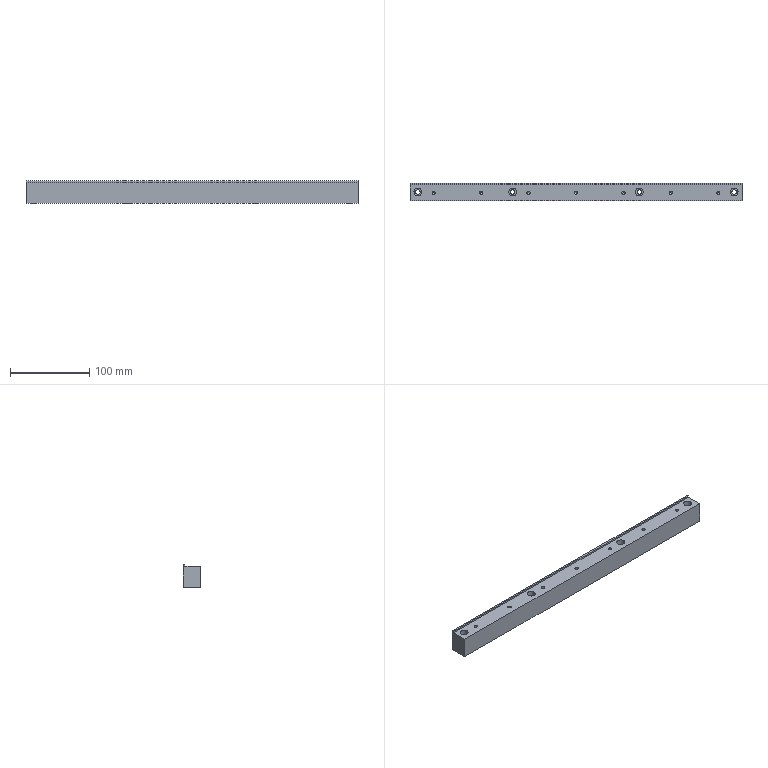Part | SolidWorks | features HoleWzd 2, Extrusion 1, ICE 1 | 1 solid | 56 faces | box 420 x 22 x 29 mm | volume 243626 mm3 | cylinder 30 | cone 14 | plane 12 | commonest cylinder face diameters 4.2 x14 5.5 x8 10 x8
STEP:
#1=CARTESIAN_POINT('',(195.,0.,10.));
#2=VERTEX_POINT('',#1);
#3=CARTESIAN_POINT('',(205.,0.,10.));
#4=VERTEX_POINT('',#3);
#5=CARTESIAN_POINT('',(200.,0.,10.));
#6=DIRECTION('',(0.,0.,1.));
#7=DIRECTION('',(1.,0.,0.));
#8=AXIS2_PLACEMENT_3D('',#5,#6,#7);
#9=CIRCLE('',#8,5.);
#10=EDGE_CURVE('',#2,#4,#9,.T.);
#11=ORIENTED_EDGE('',*,*,#10,.F.);
#12=CARTESIAN_POINT('',(195.,0.,27.));
#13=VERTEX_POINT('',#12);
#14=CARTESIAN_POINT('',(195.,0.,27.));
#15=DIRECTION('',(0.,0.,1.));
#16=VECTOR('',#15,1000.);
#17=LINE('',#14,#16);
#18=EDGE_CURVE('',#2,#13,#17,.T.);
#19=ORIENTED_EDGE('',*,*,#18,.T.);
#20=CARTESIAN_POINT('',(205.,0.,27.));
#21=VERTEX_POINT('',#20);
#22=CARTESIAN_POINT('',(200.,0.,27.));
#23=DIRECTION('',(0.,0.,1.));
#24=DIRECTION('',(1.,0.,0.));
#25=AXIS2_PLACEMENT_3D('',#22,#23,#24);
#26=CIRCLE('',#25,5.);
#27=EDGE_CURVE('',#13,#21,#26,.T.);
#28=ORIENTED_EDGE('',*,*,#27,.T.);
#29=CARTESIAN_POINT('',(205.,0.,27.));
#30=DIRECTION('',(0.,0.,1.));
#31=VECTOR('',#30,1000.);
#32=LINE('',#29,#31);
#33=EDGE_CURVE('',#4,#21,#32,.T.);
#34=ORIENTED_EDGE('',*,*,#33,.F.);
#35=EDGE_LOOP('',(#11,#19,#28,#34));
#36=FACE_OUTER_BOUND('',#35,.T.);
#37=CARTESIAN_POINT('',(200.,0.,27.));
#38=DIRECTION('',(0.,0.,1.));
#39=DIRECTION('',(1.,0.,0.));
#40=AXIS2_PLACEMENT_3D('',#37,#38,#39);
#41=CYLINDRICAL_SURFACE('',#40,5.);
#42=ADVANCED_FACE('',(#36),#41,.F.);
#43=CARTESIAN_POINT('',(197.25,0.,0.));
#44=VERTEX_POINT('',#43);
#45=CARTESIAN_POINT('',(202.75,0.,0.));
#46=VERTEX_POINT('',#45);
#47=CARTESIAN_POINT('',(200.,0.,0.));
#48=DIRECTION('',(0.,0.,1.));
#49=DIRECTION('',(1.,0.,0.));
#50=AXIS2_PLACEMENT_3D('',#47,#48,#49);
#51=CIRCLE('',#50,2.75);
#52=EDGE_CURVE('',#44,#46,#51,.T.);
#53=ORIENTED_EDGE('',*,*,#52,.F.);
#54=CARTESIAN_POINT('',(197.25,0.,10.));
#55=VERTEX_POINT('',#54);
#56=CARTESIAN_POINT('',(197.25,0.,27.));
#57=DIRECTION('',(0.,0.,1.));
#58=VECTOR('',#57,1000.);
#59=LINE('',#56,#58);
#60=EDGE_CURVE('',#44,#55,#59,.T.);
#61=ORIENTED_EDGE('',*,*,#60,.T.);
#62=CARTESIAN_POINT('',(202.75,0.,10.));
#63=VERTEX_POINT('',#62);
#64=CARTESIAN_POINT('',(200.,0.,10.));
#65=DIRECTION('',(0.,0.,1.));
#66=DIRECTION('',(1.,0.,0.));
#67=AXIS2_PLACEMENT_3D('',#64,#65,#66);
#68=CIRCLE('',#67,2.75);
#69=EDGE_CURVE('',#55,#63,#68,.T.);
#70=ORIENTED_EDGE('',*,*,#69,.T.);
#71=CARTESIAN_POINT('',(202.75,0.,27.));
#72=DIRECTION('',(0.,0.,1.));
#73=VECTOR('',#72,1000.);
#74=LINE('',#71,#73);
#75=EDGE_CURVE('',#46,#63,#74,.T.);
#76=ORIENTED_EDGE('',*,*,#75,.F.);
#77=EDGE_LOOP('',(#53,#61,#70,#76));
#78=FACE_OUTER_BOUND('',#77,.T.);
#79=CARTESIAN_POINT('',(200.,0.,27.));
#80=DIRECTION('',(0.,0.,1.));
#81=DIRECTION('',(1.,0.,0.));
#82=AXIS2_PLACEMENT_3D('',#79,#80,#81);
#83=CYLINDRICAL_SURFACE('',#82,2.75);
#84=ADVANCED_FACE('',(#78),#83,.F.);
#85=CARTESIAN_POINT('',(75.,0.,10.));
#86=VERTEX_POINT('',#85);
#87=CARTESIAN_POINT('',(85.,0.,10.));
#88=VERTEX_POINT('',#87);
#89=CARTESIAN_POINT('',(80.,0.,10.));
#90=DIRECTION('',(0.,0.,1.));
#91=DIRECTION('',(1.,0.,0.));
#92=AXIS2_PLACEMENT_3D('',#89,#90,#91);
#93=CIRCLE('',#92,5.);
#94=EDGE_CURVE('',#86,#88,#93,.T.);
#95=ORIENTED_EDGE('',*,*,#94,.F.);
#96=CARTESIAN_POINT('',(75.,0.,27.));
#97=VERTEX_POINT('',#96);
#98=CARTESIAN_POINT('',(75.,0.,27.));
#99=DIRECTION('',(0.,0.,1.));
#100=VECTOR('',#99,1000.);
#101=LINE('',#98,#100);
#102=EDGE_CURVE('',#86,#97,#101,.T.);
#103=ORIENTED_EDGE('',*,*,#102,.T.);
#104=CARTESIAN_POINT('',(85.,0.,27.));
#105=VERTEX_POINT('',#104);
#106=CARTESIAN_POINT('',(80.,0.,27.));
#107=DIRECTION('',(0.,0.,1.));
#108=DIRECTION('',(1.,0.,0.));
#109=AXIS2_PLACEMENT_3D('',#106,#107,#108);
#110=CIRCLE('',#109,5.);
#111=EDGE_CURVE('',#97,#105,#110,.T.);
#112=ORIENTED_EDGE('',*,*,#111,.T.);
#113=CARTESIAN_POINT('',(85.,0.,27.));
#114=DIRECTION('',(0.,0.,1.));
#115=VECTOR('',#114,1000.);
#116=LINE('',#113,#115);
#117=EDGE_CURVE('',#88,#105,#116,.T.);
#118=ORIENTED_EDGE('',*,*,#117,.F.);
#119=EDGE_LOOP('',(#95,#103,#112,#118));
#120=FACE_OUTER_BOUND('',#119,.T.);
#121=CARTESIAN_POINT('',(80.,0.,27.));
#122=DIRECTION('',(0.,0.,1.));
#123=DIRECTION('',(1.,0.,0.));
#124=AXIS2_PLACEMENT_3D('',#121,#122,#123);
#125=CYLINDRICAL_SURFACE('',#124,5.);
#126=ADVANCED_FACE('',(#120),#125,.F.);
#127=CARTESIAN_POINT('',(77.25,0.,0.));
#128=VERTEX_POINT('',#127);
#129=CARTESIAN_POINT('',(82.75,0.,0.));
#130=VERTEX_POINT('',#129);
#131=CARTESIAN_POINT('',(80.,0.,0.));
#132=DIRECTION('',(0.,0.,1.));
#133=DIRECTION('',(1.,0.,0.));
#134=AXIS2_PLACEMENT_3D('',#131,#132,#133);
#135=CIRCLE('',#134,2.75);
#136=EDGE_CURVE('',#128,#130,#135,.T.);
#137=ORIENTED_EDGE('',*,*,#136,.F.);
#138=CARTESIAN_POINT('',(77.25,0.,10.));
#139=VERTEX_POINT('',#138);
#140=CARTESIAN_POINT('',(77.25,0.,27.));
#141=DIRECTION('',(0.,0.,1.));
#142=VECTOR('',#141,1000.);
#143=LINE('',#140,#142);
#144=EDGE_CURVE('',#128,#139,#143,.T.);
#145=ORIENTED_EDGE('',*,*,#144,.T.);
#146=CARTESIAN_POINT('',(82.75,0.,10.));
#147=VERTEX_POINT('',#146);
#148=CARTESIAN_POINT('',(80.,0.,10.));
#149=DIRECTION('',(0.,0.,1.));
#150=DIRECTION('',(1.,0.,0.));
#151=AXIS2_PLACEMENT_3D('',#148,#149,#150);
#152=CIRCLE('',#151,2.75);
#153=EDGE_CURVE('',#139,#147,#152,.T.);
#154=ORIENTED_EDGE('',*,*,#153,.T.);
#155=CARTESIAN_POINT('',(82.75,0.,27.));
#156=DIRECTION('',(0.,0.,1.));
#157=VECTOR('',#156,1000.);
#158=LINE('',#155,#157);
#159=EDGE_CURVE('',#130,#147,#158,.T.);
#160=ORIENTED_EDGE('',*,*,#159,.F.);
#161=EDGE_LOOP('',(#137,#145,#154,#160));
#162=FACE_OUTER_BOUND('',#161,.T.);
#163=CARTESIAN_POINT('',(80.,0.,27.));
#164=DIRECTION('',(0.,0.,1.));
#165=DIRECTION('',(1.,0.,0.));
#166=AXIS2_PLACEMENT_3D('',#163,#164,#165);
#167=CYLINDRICAL_SURFACE('',#166,2.75);
#168=ADVANCED_FACE('',(#162),#167,.F.);
#169=CARTESIAN_POINT('',(-85.,0.,10.));
#170=VERTEX_POINT('',#169);
#171=CARTESIAN_POINT('',(-75.,0.,10.));
#172=VERTEX_POINT('',#171);
#173=CARTESIAN_POINT('',(-80.,0.,10.));
#174=DIRECTION('',(0.,0.,1.));
#175=DIRECTION('',(1.,0.,0.));
#176=AXIS2_PLACEMENT_3D('',#173,#174,#175);
#177=CIRCLE('',#176,5.);
#178=EDGE_CURVE('',#170,#172,#177,.T.);
#179=ORIENTED_EDGE('',*,*,#178,.F.);
#180=CARTESIAN_POINT('',(-85.,0.,27.));
#181=VERTEX_POINT('',#180);
#182=CARTESIAN_POINT('',(-85.,0.,27.));
#183=DIRECTION('',(0.,0.,1.));
#184=VECTOR('',#183,1000.);
#185=LINE('',#182,#184);
#186=EDGE_CURVE('',#170,#181,#185,.T.);
#187=ORIENTED_EDGE('',*,*,#186,.T.);
#188=CARTESIAN_POINT('',(-75.,0.,27.));
#189=VERTEX_POINT('',#188);
#190=CARTESIAN_POINT('',(-80.,0.,27.));
#191=DIRECTION('',(0.,0.,1.));
#192=DIRECTION('',(1.,0.,0.));
#193=AXIS2_PLACEMENT_3D('',#190,#191,#192);
#194=CIRCLE('',#193,5.);
#195=EDGE_CURVE('',#181,#189,#194,.T.);
#196=ORIENTED_EDGE('',*,*,#195,.T.);
#197=CARTESIAN_POINT('',(-75.,0.,27.));
#198=DIRECTION('',(0.,0.,1.));
#199=VECTOR('',#198,1000.);
#200=LINE('',#197,#199);
#201=EDGE_CURVE('',#172,#189,#200,.T.);
#202=ORIENTED_EDGE('',*,*,#201,.F.);
#203=EDGE_LOOP('',(#179,#187,#196,#202));
#204=FACE_OUTER_BOUND('',#203,.T.);
#205=CARTESIAN_POINT('',(-80.,0.,27.));
#206=DIRECTION('',(0.,0.,1.));
#207=DIRECTION('',(1.,0.,0.));
#208=AXIS2_PLACEMENT_3D('',#205,#206,#207);
#209=CYLINDRICAL_SURFACE('',#208,5.);
#210=ADVANCED_FACE('',(#204),#209,.F.);
#211=CARTESIAN_POINT('',(-82.75,0.,0.));
#212=VERTEX_POINT('',#211);
#213=CARTESIAN_POINT('',(-77.25,0.,0.));
#214=VERTEX_POINT('',#213);
#215=CARTESIAN_POINT('',(-80.,0.,0.));
#216=DIRECTION('',(0.,0.,1.));
#217=DIRECTION('',(1.,0.,0.));
#218=AXIS2_PLACEMENT_3D('',#215,#216,#217);
#219=CIRCLE('',#218,2.75);
#220=EDGE_CURVE('',#212,#214,#219,.T.);
#221=ORIENTED_EDGE('',*,*,#220,.F.);
#222=CARTESIAN_POINT('',(-82.75,0.,10.));
#223=VERTEX_POINT('',#222);
#224=CARTESIAN_POINT('',(-82.75,0.,27.));
#225=DIRECTION('',(0.,0.,1.));
#226=VECTOR('',#225,1000.);
#227=LINE('',#224,#226);
#228=EDGE_CURVE('',#212,#223,#227,.T.);
#229=ORIENTED_EDGE('',*,*,#228,.T.);
#230=CARTESIAN_POINT('',(-77.25,0.,10.));
#231=VERTEX_POINT('',#230);
#232=CARTESIAN_POINT('',(-80.,0.,10.));
#233=DIRECTION('',(0.,0.,1.));
#234=DIRECTION('',(1.,0.,0.));
#235=AXIS2_PLACEMENT_3D('',#232,#233,#234);
#236=CIRCLE('',#235,2.75);
#237=EDGE_CURVE('',#223,#231,#236,.T.);
#238=ORIENTED_EDGE('',*,*,#237,.T.);
#239=CARTESIAN_POINT('',(-77.25,0.,27.));
#240=DIRECTION('',(0.,0.,1.));
#241=VECTOR('',#240,1000.);
#242=LINE('',#239,#241);
#243=EDGE_CURVE('',#214,#231,#242,.T.);
#244=ORIENTED_EDGE('',*,*,#243,.F.);
#245=EDGE_LOOP('',(#221,#229,#238,#244));
#246=FACE_OUTER_BOUND('',#245,.T.);
#247=CARTESIAN_POINT('',(-80.,0.,27.));
#248=DIRECTION('',(0.,0.,1.));
#249=DIRECTION('',(1.,0.,0.));
#250=AXIS2_PLACEMENT_3D('',#247,#248,#249);
#251=CYLINDRICAL_SURFACE('',#250,2.75);
#252=ADVANCED_FACE('',(#246),#251,.F.);
#253=CARTESIAN_POINT('',(-205.,0.,10.));
#254=VERTEX_POINT('',#253);
#255=CARTESIAN_POINT('',(-195.,0.,10.));
#256=VERTEX_POINT('',#255);
#257=CARTESIAN_POINT('',(-200.,0.,10.));
#258=DIRECTION('',(0.,0.,1.));
#259=DIRECTION('',(1.,0.,0.));
#260=AXIS2_PLACEMENT_3D('',#257,#258,#259);
#261=CIRCLE('',#260,5.);
#262=EDGE_CURVE('',#254,#256,#261,.T.);
#263=ORIENTED_EDGE('',*,*,#262,.F.);
#264=CARTESIAN_POINT('',(-205.,0.,27.));
#265=VERTEX_POINT('',#264);
#266=CARTESIAN_POINT('',(-205.,0.,27.));
#267=DIRECTION('',(0.,0.,1.));
#268=VECTOR('',#267,1000.);
#269=LINE('',#266,#268);
#270=EDGE_CURVE('',#254,#265,#269,.T.);
#271=ORIENTED_EDGE('',*,*,#270,.T.);
#272=CARTESIAN_POINT('',(-195.,0.,27.));
#273=VERTEX_POINT('',#272);
#274=CARTESIAN_POINT('',(-200.,0.,27.));
#275=DIRECTION('',(0.,0.,1.));
#276=DIRECTION('',(1.,0.,0.));
#277=AXIS2_PLACEMENT_3D('',#274,#275,#276);
#278=CIRCLE('',#277,5.);
#279=EDGE_CURVE('',#265,#273,#278,.T.);
#280=ORIENTED_EDGE('',*,*,#279,.T.);
#281=CARTESIAN_POINT('',(-195.,0.,27.));
#282=DIRECTION('',(0.,0.,1.));
#283=VECTOR('',#282,1000.);
#284=LINE('',#281,#283);
#285=EDGE_CURVE('',#256,#273,#284,.T.);
#286=ORIENTED_EDGE('',*,*,#285,.F.);
#287=EDGE_LOOP('',(#263,#271,#280,#286));
#288=FACE_OUTER_BOUND('',#287,.T.);
#289=CARTESIAN_POINT('',(-200.,0.,27.));
#290=DIRECTION('',(0.,0.,1.));
#291=DIRECTION('',(1.,0.,0.));
#292=AXIS2_PLACEMENT_3D('',#289,#290,#291);
#293=CYLINDRICAL_SURFACE('',#292,5.);
#294=ADVANCED_FACE('',(#288),#293,.F.);
#295=CARTESIAN_POINT('',(-202.75,0.,0.));
#296=VERTEX_POINT('',#295);
#297=CARTESIAN_POINT('',(-197.25,0.,0.));
#298=VERTEX_POINT('',#297);
#299=CARTESIAN_POINT('',(-200.,0.,0.));
#300=DIRECTION('',(0.,0.,1.));
#301=DIRECTION('',(1.,0.,0.));
#302=AXIS2_PLACEMENT_3D('',#299,#300,#301);
#303=CIRCLE('',#302,2.75);
#304=EDGE_CURVE('',#296,#298,#303,.T.);
#305=ORIENTED_EDGE('',*,*,#304,.F.);
#306=CARTESIAN_POINT('',(-202.75,0.,10.));
#307=VERTEX_POINT('',#306);
#308=CARTESIAN_POINT('',(-202.75,0.,27.));
#309=DIRECTION('',(0.,0.,1.));
#310=VECTOR('',#309,1000.);
#311=LINE('',#308,#310);
#312=EDGE_CURVE('',#296,#307,#311,.T.);
#313=ORIENTED_EDGE('',*,*,#312,.T.);
#314=CARTESIAN_POINT('',(-197.25,0.,10.));
#315=VERTEX_POINT('',#314);
#316=CARTESIAN_POINT('',(-200.,0.,10.));
#317=DIRECTION('',(0.,0.,1.));
#318=DIRECTION('',(1.,0.,0.));
#319=AXIS2_PLACEMENT_3D('',#316,#317,#318);
#320=CIRCLE('',#319,2.75);
#321=EDGE_CURVE('',#307,#315,#320,.T.);
#322=ORIENTED_EDGE('',*,*,#321,.T.);
#323=CARTESIAN_POINT('',(-197.25,0.,27.));
#324=DIRECTION('',(0.,0.,1.));
#325=VECTOR('',#324,1000.);
#326=LINE('',#323,#325);
#327=EDGE_CURVE('',#298,#315,#326,.T.);
#328=ORIENTED_EDGE('',*,*,#327,.F.);
#329=EDGE_LOOP('',(#305,#313,#322,#328));
#330=FACE_OUTER_BOUND('',#329,.T.);
#331=CARTESIAN_POINT('',(-200.,0.,27.));
#332=DIRECTION('',(0.,0.,1.));
#333=DIRECTION('',(1.,0.,0.));
#334=AXIS2_PLACEMENT_3D('',#331,#332,#333);
#335=CYLINDRICAL_SURFACE('',#334,2.75);
#336=ADVANCED_FACE('',(#330),#335,.F.);
#337=CARTESIAN_POINT('',(177.9,-1.,14.6));
#338=VERTEX_POINT('',#337);
#339=CARTESIAN_POINT('',(182.1,-1.,14.6));
#340=VERTEX_POINT('',#339);
#341=CARTESIAN_POINT('',(180.,-1.,14.6));
#342=DIRECTION('',(0.,0.,1.));
#343=DIRECTION('',(1.,0.,0.));
#344=AXIS2_PLACEMENT_3D('',#341,#342,#343);
#345=CIRCLE('',#344,2.1);
#346=EDGE_CURVE('',#338,#340,#345,.T.);
#347=ORIENTED_EDGE('',*,*,#346,.F.);
#348=CARTESIAN_POINT('',(177.9,-1.,27.));
#349=VERTEX_POINT('',#348);
#350=CARTESIAN_POINT('',(177.9,-1.,27.));
#351=DIRECTION('',(0.,0.,1.));
#352=VECTOR('',#351,1000.);
#353=LINE('',#350,#352);
#354=EDGE_CURVE('',#338,#349,#353,.T.);
#355=ORIENTED_EDGE('',*,*,#354,.T.);
#356=CARTESIAN_POINT('',(182.1,-1.,27.));
#357=VERTEX_POINT('',#356);
#358=CARTESIAN_POINT('',(180.,-1.,27.));
#359=DIRECTION('',(0.,0.,1.));
#360=DIRECTION('',(1.,0.,0.));
#361=AXIS2_PLACEMENT_3D('',#358,#359,#360);
#362=CIRCLE('',#361,2.1);
#363=EDGE_CURVE('',#349,#357,#362,.T.);
#364=ORIENTED_EDGE('',*,*,#363,.T.);
#365=CARTESIAN_POINT('',(182.1,-1.,27.));
#366=DIRECTION('',(0.,0.,1.));
#367=VECTOR('',#366,1000.);
#368=LINE('',#365,#367);
#369=EDGE_CURVE('',#340,#357,#368,.T.);
#370=ORIENTED_EDGE('',*,*,#369,.F.);
#371=EDGE_LOOP('',(#347,#355,#364,#370));
#372=FACE_OUTER_BOUND('',#371,.T.);
#373=CARTESIAN_POINT('',(180.,-1.,27.));
#374=DIRECTION('',(0.,0.,1.));
#375=DIRECTION('',(1.,0.,0.));
#376=AXIS2_PLACEMENT_3D('',#373,#374,#375);
#377=CYLINDRICAL_SURFACE('',#376,2.1);
#378=ADVANCED_FACE('',(#372),#377,.F.);
#379=CARTESIAN_POINT('',(180.,-1.,13.338));
#380=VERTEX_POINT('',#379);
#381=CARTESIAN_POINT('',(182.1,-1.,14.6));
#382=DIRECTION('',(0.8572,0.,0.515));
#383=VECTOR('',#382,1000.);
#384=LINE('',#381,#383);
#385=EDGE_CURVE('',#380,#340,#384,.T.);
#386=ORIENTED_EDGE('',*,*,#385,.F.);
#387=CARTESIAN_POINT('',(177.9,-1.,14.6));
#388=DIRECTION('',(-0.8572,0.,0.515));
#389=VECTOR('',#388,1000.);
#390=LINE('',#387,#389);
#391=EDGE_CURVE('',#380,#338,#390,.T.);
#392=ORIENTED_EDGE('',*,*,#391,.T.);
#393=ORIENTED_EDGE('',*,*,#346,.T.);
#394=EDGE_LOOP('',(#386,#392,#393));
#395=FACE_OUTER_BOUND('',#394,.T.);
#396=CARTESIAN_POINT('',(180.,-1.,14.6));
#397=DIRECTION('',(0.,0.,1.));
#398=DIRECTION('',(1.,0.,0.));
#399=AXIS2_PLACEMENT_3D('',#396,#397,#398);
#400=CONICAL_SURFACE('',#399,2.1,1.03);
#401=ADVANCED_FACE('',(#395),#400,.F.);
#402=CARTESIAN_POINT('',(117.9,-1.,14.6));
#403=VERTEX_POINT('',#402);
#404=CARTESIAN_POINT('',(122.1,-1.,14.6));
#405=VERTEX_POINT('',#404);
#406=CARTESIAN_POINT('',(120.,-1.,14.6));
#407=DIRECTION('',(0.,0.,1.));
#408=DIRECTION('',(1.,0.,0.));
#409=AXIS2_PLACEMENT_3D('',#406,#407,#408);
#410=CIRCLE('',#409,2.1);
#411=EDGE_CURVE('',#403,#405,#410,.T.);
#412=ORIENTED_EDGE('',*,*,#411,.F.);
#413=CARTESIAN_POINT('',(117.9,-1.,27.));
#414=VERTEX_POINT('',#413);
#415=CARTESIAN_POINT('',(117.9,-1.,27.));
#416=DIRECTION('',(0.,0.,1.));
#417=VECTOR('',#416,1000.);
#418=LINE('',#415,#417);
#419=EDGE_CURVE('',#403,#414,#418,.T.);
#420=ORIENTED_EDGE('',*,*,#419,.T.);
#421=CARTESIAN_POINT('',(122.1,-1.,27.));
#422=VERTEX_POINT('',#421);
#423=CARTESIAN_POINT('',(120.,-1.,27.));
#424=DIRECTION('',(0.,0.,1.));
#425=DIRECTION('',(1.,0.,0.));
#426=AXIS2_PLACEMENT_3D('',#423,#424,#425);
#427=CIRCLE('',#426,2.1);
#428=EDGE_CURVE('',#414,#422,#427,.T.);
#429=ORIENTED_EDGE('',*,*,#428,.T.);
#430=CARTESIAN_POINT('',(122.1,-1.,27.));
#431=DIRECTION('',(0.,0.,1.));
#432=VECTOR('',#431,1000.);
#433=LINE('',#430,#432);
#434=EDGE_CURVE('',#405,#422,#433,.T.);
#435=ORIENTED_EDGE('',*,*,#434,.F.);
#436=EDGE_LOOP('',(#412,#420,#429,#435));
#437=FACE_OUTER_BOUND('',#436,.T.);
#438=CARTESIAN_POINT('',(120.,-1.,27.));
#439=DIRECTION('',(0.,0.,1.));
#440=DIRECTION('',(1.,0.,0.));
#441=AXIS2_PLACEMENT_3D('',#438,#439,#440);
#442=CYLINDRICAL_SURFACE('',#441,2.1);
#443=ADVANCED_FACE('',(#437),#442,.F.);
#444=CARTESIAN_POINT('',(120.,-1.,13.338));
#445=VERTEX_POINT('',#444);
#446=CARTESIAN_POINT('',(122.1,-1.,14.6));
#447=DIRECTION('',(0.8572,0.,0.515));
#448=VECTOR('',#447,1000.);
#449=LINE('',#446,#448);
#450=EDGE_CURVE('',#445,#405,#449,.T.);
#451=ORIENTED_EDGE('',*,*,#450,.F.);
#452=CARTESIAN_POINT('',(117.9,-1.,14.6));
#453=DIRECTION('',(-0.8572,0.,0.515));
#454=VECTOR('',#453,1000.);
#455=LINE('',#452,#454);
#456=EDGE_CURVE('',#445,#403,#455,.T.);
#457=ORIENTED_EDGE('',*,*,#456,.T.);
#458=ORIENTED_EDGE('',*,*,#411,.T.);
#459=EDGE_LOOP('',(#451,#457,#458));
#460=FACE_OUTER_BOUND('',#459,.T.);
#461=CARTESIAN_POINT('',(120.,-1.,14.6));
#462=DIRECTION('',(0.,0.,1.));
#463=DIRECTION('',(1.,0.,0.));
#464=AXIS2_PLACEMENT_3D('',#461,#462,#463);
#465=CONICAL_SURFACE('',#464,2.1,1.03);
#466=ADVANCED_FACE('',(#460),#465,.F.);
#467=CARTESIAN_POINT('',(57.9,-1.,14.6));
#468=VERTEX_POINT('',#467);
#469=CARTESIAN_POINT('',(62.1,-1.,14.6));
#470=VERTEX_POINT('',#469);
#471=CARTESIAN_POINT('',(60.,-1.,14.6));
#472=DIRECTION('',(0.,0.,1.));
#473=DIRECTION('',(1.,0.,0.));
#474=AXIS2_PLACEMENT_3D('',#471,#472,#473);
#475=CIRCLE('',#474,2.1);
#476=EDGE_CURVE('',#468,#470,#475,.T.);
#477=ORIENTED_EDGE('',*,*,#476,.F.);
#478=CARTESIAN_POINT('',(57.9,-1.,27.));
#479=VERTEX_POINT('',#478);
#480=CARTESIAN_POINT('',(57.9,-1.,27.));
#481=DIRECTION('',(0.,0.,1.));
#482=VECTOR('',#481,1000.);
#483=LINE('',#480,#482);
#484=EDGE_CURVE('',#468,#479,#483,.T.);
#485=ORIENTED_EDGE('',*,*,#484,.T.);
#486=CARTESIAN_POINT('',(62.1,-1.,27.));
#487=VERTEX_POINT('',#486);
#488=CARTESIAN_POINT('',(60.,-1.,27.));
#489=DIRECTION('',(0.,0.,1.));
#490=DIRECTION('',(1.,0.,0.));
#491=AXIS2_PLACEMENT_3D('',#488,#489,#490);
#492=CIRCLE('',#491,2.1);
#493=EDGE_CURVE('',#479,#487,#492,.T.);
#494=ORIENTED_EDGE('',*,*,#493,.T.);
#495=CARTESIAN_POINT('',(62.1,-1.,27.));
#496=DIRECTION('',(0.,0.,1.));
#497=VECTOR('',#496,1000.);
#498=LINE('',#495,#497);
#499=EDGE_CURVE('',#470,#487,#498,.T.);
#500=ORIENTED_EDGE('',*,*,#499,.F.);
#501=EDGE_LOOP('',(#477,#485,#494,#500));
#502=FACE_OUTER_BOUND('',#501,.T.);
#503=CARTESIAN_POINT('',(60.,-1.,27.));
#504=DIRECTION('',(0.,0.,1.));
#505=DIRECTION('',(1.,0.,0.));
#506=AXIS2_PLACEMENT_3D('',#503,#504,#505);
#507=CYLINDRICAL_SURFACE('',#506,2.1);
#508=ADVANCED_FACE('',(#502),#507,.F.);
#509=CARTESIAN_POINT('',(60.,-1.,13.338));
#510=VERTEX_POINT('',#509);
#511=CARTESIAN_POINT('',(62.1,-1.,14.6));
#512=DIRECTION('',(0.8572,0.,0.515));
#513=VECTOR('',#512,1000.);
#514=LINE('',#511,#513);
#515=EDGE_CURVE('',#510,#470,#514,.T.);
#516=ORIENTED_EDGE('',*,*,#515,.F.);
#517=CARTESIAN_POINT('',(57.9,-1.,14.6));
#518=DIRECTION('',(-0.8572,0.,0.515));
#519=VECTOR('',#518,1000.);
#520=LINE('',#517,#519);
#521=EDGE_CURVE('',#510,#468,#520,.T.);
#522=ORIENTED_EDGE('',*,*,#521,.T.);
#523=ORIENTED_EDGE('',*,*,#476,.T.);
#524=EDGE_LOOP('',(#516,#522,#523));
#525=FACE_OUTER_BOUND('',#524,.T.);
#526=CARTESIAN_POINT('',(60.,-1.,14.6));
#527=DIRECTION('',(0.,0.,1.));
#528=DIRECTION('',(1.,0.,0.));
#529=AXIS2_PLACEMENT_3D('',#526,#527,#528);
#530=CONICAL_SURFACE('',#529,2.1,1.03);
#531=ADVANCED_FACE('',(#525),#530,.F.);
#532=CARTESIAN_POINT('',(-2.1,-1.,14.6));
#533=VERTEX_POINT('',#532);
#534=CARTESIAN_POINT('',(2.1,-1.,14.6));
#535=VERTEX_POINT('',#534);
#536=CARTESIAN_POINT('',(0.,-1.,14.6));
#537=DIRECTION('',(0.,0.,1.));
#538=DIRECTION('',(1.,0.,0.));
#539=AXIS2_PLACEMENT_3D('',#536,#537,#538);
#540=CIRCLE('',#539,2.1);
#541=EDGE_CURVE('',#533,#535,#540,.T.);
#542=ORIENTED_EDGE('',*,*,#541,.F.);
#543=CARTESIAN_POINT('',(-2.1,-1.,27.));
#544=VERTEX_POINT('',#543);
#545=CARTESIAN_POINT('',(-2.1,-1.,27.));
#546=DIRECTION('',(0.,0.,1.));
#547=VECTOR('',#546,1000.);
#548=LINE('',#545,#547);
#549=EDGE_CURVE('',#533,#544,#548,.T.);
#550=ORIENTED_EDGE('',*,*,#549,.T.);
#551=CARTESIAN_POINT('',(2.1,-1.,27.));
#552=VERTEX_POINT('',#551);
#553=CARTESIAN_POINT('',(0.,-1.,27.));
#554=DIRECTION('',(0.,0.,1.));
#555=DIRECTION('',(1.,0.,0.));
#556=AXIS2_PLACEMENT_3D('',#553,#554,#555);
#557=CIRCLE('',#556,2.1);
#558=EDGE_CURVE('',#544,#552,#557,.T.);
#559=ORIENTED_EDGE('',*,*,#558,.T.);
#560=CARTESIAN_POINT('',(2.1,-1.,27.));
#561=DIRECTION('',(0.,0.,1.));
#562=VECTOR('',#561,1000.);
#563=LINE('',#560,#562);
#564=EDGE_CURVE('',#535,#552,#563,.T.);
#565=ORIENTED_EDGE('',*,*,#564,.F.);
#566=EDGE_LOOP('',(#542,#550,#559,#565));
#567=FACE_OUTER_BOUND('',#566,.T.);
#568=CARTESIAN_POINT('',(0.,-1.,27.));
#569=DIRECTION('',(0.,0.,1.));
#570=DIRECTION('',(1.,0.,0.));
#571=AXIS2_PLACEMENT_3D('',#568,#569,#570);
#572=CYLINDRICAL_SURFACE('',#571,2.1);
#573=ADVANCED_FACE('',(#567),#572,.F.);
#574=CARTESIAN_POINT('',(0.,-1.,13.338));
#575=VERTEX_POINT('',#574);
#576=CARTESIAN_POINT('',(2.1,-1.,14.6));
#577=DIRECTION('',(0.8572,0.,0.515));
#578=VECTOR('',#577,1000.);
#579=LINE('',#576,#578);
#580=EDGE_CURVE('',#575,#535,#579,.T.);
#581=ORIENTED_EDGE('',*,*,#580,.F.);
#582=CARTESIAN_POINT('',(-2.1,-1.,14.6));
#583=DIRECTION('',(-0.8572,0.,0.515));
#584=VECTOR('',#583,1000.);
#585=LINE('',#582,#584);
#586=EDGE_CURVE('',#575,#533,#585,.T.);
#587=ORIENTED_EDGE('',*,*,#586,.T.);
#588=ORIENTED_EDGE('',*,*,#541,.T.);
#589=EDGE_LOOP('',(#581,#587,#588));
#590=FACE_OUTER_BOUND('',#589,.T.);
#591=CARTESIAN_POINT('',(0.,-1.,14.6));
#592=DIRECTION('',(0.,0.,1.));
#593=DIRECTION('',(1.,0.,0.));
#594=AXIS2_PLACEMENT_3D('',#591,#592,#593);
#595=CONICAL_SURFACE('',#594,2.1,1.03);
#596=ADVANCED_FACE('',(#590),#595,.F.);
#597=CARTESIAN_POINT('',(-182.1,-1.,14.6));
#598=VERTEX_POINT('',#597);
#599=CARTESIAN_POINT('',(-177.9,-1.,14.6));
#600=VERTEX_POINT('',#599);
#601=CARTESIAN_POINT('',(-180.,-1.,14.6));
#602=DIRECTION('',(0.,0.,1.));
#603=DIRECTION('',(1.,0.,0.));
#604=AXIS2_PLACEMENT_3D('',#601,#602,#603);
#605=CIRCLE('',#604,2.1);
#606=EDGE_CURVE('',#598,#600,#605,.T.);
#607=ORIENTED_EDGE('',*,*,#606,.F.);
#608=CARTESIAN_POINT('',(-182.1,-1.,27.));
#609=VERTEX_POINT('',#608);
#610=CARTESIAN_POINT('',(-182.1,-1.,27.));
#611=DIRECTION('',(0.,0.,1.));
#612=VECTOR('',#611,1000.);
#613=LINE('',#610,#612);
#614=EDGE_CURVE('',#598,#609,#613,.T.);
#615=ORIENTED_EDGE('',*,*,#614,.T.);
#616=CARTESIAN_POINT('',(-177.9,-1.,27.));
#617=VERTEX_POINT('',#616);
#618=CARTESIAN_POINT('',(-180.,-1.,27.));
#619=DIRECTION('',(0.,0.,1.));
#620=DIRECTION('',(1.,0.,0.));
#621=AXIS2_PLACEMENT_3D('',#618,#619,#620);
#622=CIRCLE('',#621,2.1);
#623=EDGE_CURVE('',#609,#617,#622,.T.);
#624=ORIENTED_EDGE('',*,*,#623,.T.);
#625=CARTESIAN_POINT('',(-177.9,-1.,27.));
#626=DIRECTION('',(0.,0.,1.));
#627=VECTOR('',#626,1000.);
#628=LINE('',#625,#627);
#629=EDGE_CURVE('',#600,#617,#628,.T.);
#630=ORIENTED_EDGE('',*,*,#629,.F.);
#631=EDGE_LOOP('',(#607,#615,#624,#630));
#632=FACE_OUTER_BOUND('',#631,.T.);
#633=CARTESIAN_POINT('',(-180.,-1.,27.));
#634=DIRECTION('',(0.,0.,1.));
#635=DIRECTION('',(1.,0.,0.));
#636=AXIS2_PLACEMENT_3D('',#633,#634,#635);
#637=CYLINDRICAL_SURFACE('',#636,2.1);
#638=ADVANCED_FACE('',(#632),#637,.F.);
#639=CARTESIAN_POINT('',(-180.,-1.,13.338));
#640=VERTEX_POINT('',#639);
#641=CARTESIAN_POINT('',(-177.9,-1.,14.6));
#642=DIRECTION('',(0.8572,0.,0.515));
#643=VECTOR('',#642,1000.);
#644=LINE('',#641,#643);
#645=EDGE_CURVE('',#640,#600,#644,.T.);
#646=ORIENTED_EDGE('',*,*,#645,.F.);
#647=CARTESIAN_POINT('',(-182.1,-1.,14.6));
#648=DIRECTION('',(-0.8572,0.,0.515));
#649=VECTOR('',#648,1000.);
#650=LINE('',#647,#649);
#651=EDGE_CURVE('',#640,#598,#650,.T.);
#652=ORIENTED_EDGE('',*,*,#651,.T.);
#653=ORIENTED_EDGE('',*,*,#606,.T.);
#654=EDGE_LOOP('',(#646,#652,#653));
#655=FACE_OUTER_BOUND('',#654,.T.);
#656=CARTESIAN_POINT('',(-180.,-1.,14.6));
#657=DIRECTION('',(0.,0.,1.));
#658=DIRECTION('',(1.,0.,0.));
#659=AXIS2_PLACEMENT_3D('',#656,#657,#658);
#660=CONICAL_SURFACE('',#659,2.1,1.03);
#661=ADVANCED_FACE('',(#655),#660,.F.);
#662=CARTESIAN_POINT('',(-122.1,-1.,14.6));
#663=VERTEX_POINT('',#662);
#664=CARTESIAN_POINT('',(-117.9,-1.,14.6));
#665=VERTEX_POINT('',#664);
#666=CARTESIAN_POINT('',(-120.,-1.,14.6));
#667=DIRECTION('',(0.,0.,1.));
#668=DIRECTION('',(1.,0.,0.));
#669=AXIS2_PLACEMENT_3D('',#666,#667,#668);
#670=CIRCLE('',#669,2.1);
#671=EDGE_CURVE('',#663,#665,#670,.T.);
#672=ORIENTED_EDGE('',*,*,#671,.F.);
#673=CARTESIAN_POINT('',(-122.1,-1.,27.));
#674=VERTEX_POINT('',#673);
#675=CARTESIAN_POINT('',(-122.1,-1.,27.));
#676=DIRECTION('',(0.,0.,1.));
#677=VECTOR('',#676,1000.);
#678=LINE('',#675,#677);
#679=EDGE_CURVE('',#663,#674,#678,.T.);
#680=ORIENTED_EDGE('',*,*,#679,.T.);
#681=CARTESIAN_POINT('',(-117.9,-1.,27.));
#682=VERTEX_POINT('',#681);
#683=CARTESIAN_POINT('',(-120.,-1.,27.));
#684=DIRECTION('',(0.,0.,1.));
#685=DIRECTION('',(1.,0.,0.));
#686=AXIS2_PLACEMENT_3D('',#683,#684,#685);
#687=CIRCLE('',#686,2.1);
#688=EDGE_CURVE('',#674,#682,#687,.T.);
#689=ORIENTED_EDGE('',*,*,#688,.T.);
#690=CARTESIAN_POINT('',(-117.9,-1.,27.));
#691=DIRECTION('',(0.,0.,1.));
#692=VECTOR('',#691,1000.);
#693=LINE('',#690,#692);
#694=EDGE_CURVE('',#665,#682,#693,.T.);
#695=ORIENTED_EDGE('',*,*,#694,.F.);
#696=EDGE_LOOP('',(#672,#680,#689,#695));
#697=FACE_OUTER_BOUND('',#696,.T.);
#698=CARTESIAN_POINT('',(-120.,-1.,27.));
#699=DIRECTION('',(0.,0.,1.));
#700=DIRECTION('',(1.,0.,0.));
#701=AXIS2_PLACEMENT_3D('',#698,#699,#700);
#702=CYLINDRICAL_SURFACE('',#701,2.1);
#703=ADVANCED_FACE('',(#697),#702,.F.);
#704=CARTESIAN_POINT('',(-120.,-1.,13.338));
#705=VERTEX_POINT('',#704);
#706=CARTESIAN_POINT('',(-117.9,-1.,14.6));
#707=DIRECTION('',(0.8572,0.,0.515));
#708=VECTOR('',#707,1000.);
#709=LINE('',#706,#708);
#710=EDGE_CURVE('',#705,#665,#709,.T.);
#711=ORIENTED_EDGE('',*,*,#710,.F.);
#712=CARTESIAN_POINT('',(-122.1,-1.,14.6));
#713=DIRECTION('',(-0.8572,0.,0.515));
#714=VECTOR('',#713,1000.);
#715=LINE('',#712,#714);
#716=EDGE_CURVE('',#705,#663,#715,.T.);
#717=ORIENTED_EDGE('',*,*,#716,.T.);
#718=ORIENTED_EDGE('',*,*,#671,.T.);
#719=EDGE_LOOP('',(#711,#717,#718));
#720=FACE_OUTER_BOUND('',#719,.T.);
#721=CARTESIAN_POINT('',(-120.,-1.,14.6));
#722=DIRECTION('',(0.,0.,1.));
#723=DIRECTION('',(1.,0.,0.));
#724=AXIS2_PLACEMENT_3D('',#721,#722,#723);
#725=CONICAL_SURFACE('',#724,2.1,1.03);
#726=ADVANCED_FACE('',(#720),#725,.F.);
#727=CARTESIAN_POINT('',(-62.1,-1.,14.6));
#728=VERTEX_POINT('',#727);
#729=CARTESIAN_POINT('',(-57.9,-1.,14.6));
#730=VERTEX_POINT('',#729);
#731=CARTESIAN_POINT('',(-60.,-1.,14.6));
#732=DIRECTION('',(0.,0.,1.));
#733=DIRECTION('',(1.,0.,0.));
#734=AXIS2_PLACEMENT_3D('',#731,#732,#733);
#735=CIRCLE('',#734,2.1);
#736=EDGE_CURVE('',#728,#730,#735,.T.);
#737=ORIENTED_EDGE('',*,*,#736,.F.);
#738=CARTESIAN_POINT('',(-62.1,-1.,27.));
#739=VERTEX_POINT('',#738);
#740=CARTESIAN_POINT('',(-62.1,-1.,27.));
#741=DIRECTION('',(0.,0.,1.));
#742=VECTOR('',#741,1000.);
#743=LINE('',#740,#742);
#744=EDGE_CURVE('',#728,#739,#743,.T.);
#745=ORIENTED_EDGE('',*,*,#744,.T.);
#746=CARTESIAN_POINT('',(-57.9,-1.,27.));
#747=VERTEX_POINT('',#746);
#748=CARTESIAN_POINT('',(-60.,-1.,27.));
#749=DIRECTION('',(0.,0.,1.));
#750=DIRECTION('',(1.,0.,0.));
#751=AXIS2_PLACEMENT_3D('',#748,#749,#750);
#752=CIRCLE('',#751,2.1);
#753=EDGE_CURVE('',#739,#747,#752,.T.);
#754=ORIENTED_EDGE('',*,*,#753,.T.);
#755=CARTESIAN_POINT('',(-57.9,-1.,27.));
#756=DIRECTION('',(0.,0.,1.));
#757=VECTOR('',#756,1000.);
#758=LINE('',#755,#757);
#759=EDGE_CURVE('',#730,#747,#758,.T.);
#760=ORIENTED_EDGE('',*,*,#759,.F.);
#761=EDGE_LOOP('',(#737,#745,#754,#760));
#762=FACE_OUTER_BOUND('',#761,.T.);
#763=CARTESIAN_POINT('',(-60.,-1.,27.));
#764=DIRECTION('',(0.,0.,1.));
#765=DIRECTION('',(1.,0.,0.));
#766=AXIS2_PLACEMENT_3D('',#763,#764,#765);
#767=CYLINDRICAL_SURFACE('',#766,2.1);
#768=ADVANCED_FACE('',(#762),#767,.F.);
#769=CARTESIAN_POINT('',(-60.,-1.,13.338));
#770=VERTEX_POINT('',#769);
#771=CARTESIAN_POINT('',(-57.9,-1.,14.6));
#772=DIRECTION('',(0.8572,0.,0.515));
#773=VECTOR('',#772,1000.);
#774=LINE('',#771,#773);
#775=EDGE_CURVE('',#770,#730,#774,.T.);
#776=ORIENTED_EDGE('',*,*,#775,.F.);
#777=CARTESIAN_POINT('',(-62.1,-1.,14.6));
#778=DIRECTION('',(-0.8572,0.,0.515));
#779=VECTOR('',#778,1000.);
#780=LINE('',#777,#779);
#781=EDGE_CURVE('',#770,#728,#780,.T.);
#782=ORIENTED_EDGE('',*,*,#781,.T.);
#783=ORIENTED_EDGE('',*,*,#736,.T.);
#784=EDGE_LOOP('',(#776,#782,#783));
#785=FACE_OUTER_BOUND('',#784,.T.);
#786=CARTESIAN_POINT('',(-60.,-1.,14.6));
#787=DIRECTION('',(0.,0.,1.));
#788=DIRECTION('',(1.,0.,0.));
#789=AXIS2_PLACEMENT_3D('',#786,#787,#788);
#790=CONICAL_SURFACE('',#789,2.1,1.03);
#791=ADVANCED_FACE('',(#785),#790,.F.);
#792=CARTESIAN_POINT('',(200.,0.,27.));
#793=DIRECTION('',(0.,0.,1.));
#794=DIRECTION('',(1.,0.,0.));
#795=AXIS2_PLACEMENT_3D('',#792,#793,#794);
#796=CIRCLE('',#795,5.);
#797=EDGE_CURVE('',#21,#13,#796,.T.);
#798=ORIENTED_EDGE('',*,*,#797,.F.);
#799=ORIENTED_EDGE('',*,*,#27,.F.);
#800=EDGE_LOOP('',(#798,#799));
#801=FACE_BOUND('',#800,.T.);
#802=CARTESIAN_POINT('',(80.,0.,27.));
#803=DIRECTION('',(0.,0.,1.));
#804=DIRECTION('',(1.,0.,0.));
#805=AXIS2_PLACEMENT_3D('',#802,#803,#804);
#806=CIRCLE('',#805,5.);
#807=EDGE_CURVE('',#105,#97,#806,.T.);
#808=ORIENTED_EDGE('',*,*,#807,.F.);
#809=ORIENTED_EDGE('',*,*,#111,.F.);
#810=EDGE_LOOP('',(#808,#809));
#811=FACE_BOUND('',#810,.T.);
#812=CARTESIAN_POINT('',(-80.,0.,27.));
#813=DIRECTION('',(0.,0.,1.));
#814=DIRECTION('',(1.,0.,0.));
#815=AXIS2_PLACEMENT_3D('',#812,#813,#814);
#816=CIRCLE('',#815,5.);
#817=EDGE_CURVE('',#189,#181,#816,.T.);
#818=ORIENTED_EDGE('',*,*,#817,.F.);
#819=ORIENTED_EDGE('',*,*,#195,.F.);
#820=EDGE_LOOP('',(#818,#819));
#821=FACE_BOUND('',#820,.T.);
#822=CARTESIAN_POINT('',(-200.,0.,27.));
#823=DIRECTION('',(0.,0.,1.));
#824=DIRECTION('',(1.,0.,0.));
#825=AXIS2_PLACEMENT_3D('',#822,#823,#824);
#826=CIRCLE('',#825,5.);
#827=EDGE_CURVE('',#273,#265,#826,.T.);
#828=ORIENTED_EDGE('',*,*,#827,.F.);
#829=ORIENTED_EDGE('',*,*,#279,.F.);
#830=EDGE_LOOP('',(#828,#829));
#831=FACE_BOUND('',#830,.T.);
#832=CARTESIAN_POINT('',(180.,-1.,27.));
#833=DIRECTION('',(0.,0.,1.));
#834=DIRECTION('',(1.,0.,0.));
#835=AXIS2_PLACEMENT_3D('',#832,#833,#834);
#836=CIRCLE('',#835,2.1);
#837=EDGE_CURVE('',#357,#349,#836,.T.);
#838=ORIENTED_EDGE('',*,*,#837,.F.);
#839=ORIENTED_EDGE('',*,*,#363,.F.);
#840=EDGE_LOOP('',(#838,#839));
#841=FACE_BOUND('',#840,.T.);
#842=CARTESIAN_POINT('',(120.,-1.,27.));
#843=DIRECTION('',(0.,0.,1.));
#844=DIRECTION('',(1.,0.,0.));
#845=AXIS2_PLACEMENT_3D('',#842,#843,#844);
#846=CIRCLE('',#845,2.1);
#847=EDGE_CURVE('',#422,#414,#846,.T.);
#848=ORIENTED_EDGE('',*,*,#847,.F.);
#849=ORIENTED_EDGE('',*,*,#428,.F.);
#850=EDGE_LOOP('',(#848,#849));
#851=FACE_BOUND('',#850,.T.);
#852=CARTESIAN_POINT('',(60.,-1.,27.));
#853=DIRECTION('',(0.,0.,1.));
#854=DIRECTION('',(1.,0.,0.));
#855=AXIS2_PLACEMENT_3D('',#852,#853,#854);
#856=CIRCLE('',#855,2.1);
#857=EDGE_CURVE('',#487,#479,#856,.T.);
#858=ORIENTED_EDGE('',*,*,#857,.F.);
#859=ORIENTED_EDGE('',*,*,#493,.F.);
#860=EDGE_LOOP('',(#858,#859));
#861=FACE_BOUND('',#860,.T.);
#862=CARTESIAN_POINT('',(0.,-1.,27.));
#863=DIRECTION('',(0.,0.,1.));
#864=DIRECTION('',(1.,0.,0.));
#865=AXIS2_PLACEMENT_3D('',#862,#863,#864);
#866=CIRCLE('',#865,2.1);
#867=EDGE_CURVE('',#552,#544,#866,.T.);
#868=ORIENTED_EDGE('',*,*,#867,.F.);
#869=ORIENTED_EDGE('',*,*,#558,.F.);
#870=EDGE_LOOP('',(#868,#869));
#871=FACE_BOUND('',#870,.T.);
#872=CARTESIAN_POINT('',(-180.,-1.,27.));
#873=DIRECTION('',(0.,0.,1.));
#874=DIRECTION('',(1.,0.,0.));
#875=AXIS2_PLACEMENT_3D('',#872,#873,#874);
#876=CIRCLE('',#875,2.1);
#877=EDGE_CURVE('',#617,#609,#876,.T.);
#878=ORIENTED_EDGE('',*,*,#877,.F.);
#879=ORIENTED_EDGE('',*,*,#623,.F.);
#880=EDGE_LOOP('',(#878,#879));
#881=FACE_BOUND('',#880,.T.);
#882=CARTESIAN_POINT('',(-120.,-1.,27.));
#883=DIRECTION('',(0.,0.,1.));
#884=DIRECTION('',(1.,0.,0.));
#885=AXIS2_PLACEMENT_3D('',#882,#883,#884);
#886=CIRCLE('',#885,2.1);
#887=EDGE_CURVE('',#682,#674,#886,.T.);
#888=ORIENTED_EDGE('',*,*,#887,.F.);
#889=ORIENTED_EDGE('',*,*,#688,.F.);
#890=EDGE_LOOP('',(#888,#889));
#891=FACE_BOUND('',#890,.T.);
#892=CARTESIAN_POINT('',(-60.,-1.,27.));
#893=DIRECTION('',(0.,0.,1.));
#894=DIRECTION('',(1.,0.,0.));
#895=AXIS2_PLACEMENT_3D('',#892,#893,#894);
#896=CIRCLE('',#895,2.1);
#897=EDGE_CURVE('',#747,#739,#896,.T.);
#898=ORIENTED_EDGE('',*,*,#897,.F.);
#899=ORIENTED_EDGE('',*,*,#753,.F.);
#900=EDGE_LOOP('',(#898,#899));
#901=FACE_BOUND('',#900,.T.);
#902=CARTESIAN_POINT('',(-210.,9.,27.));
#903=VERTEX_POINT('',#902);
#904=CARTESIAN_POINT('',(210.,9.,27.));
#905=VERTEX_POINT('',#904);
#906=CARTESIAN_POINT('',(-210.,9.,27.));
#907=DIRECTION('',(1.,0.,0.));
#908=VECTOR('',#907,1000.);
#909=LINE('',#906,#908);
#910=EDGE_CURVE('',#903,#905,#909,.T.);
#911=ORIENTED_EDGE('',*,*,#910,.F.);
#912=CARTESIAN_POINT('',(-210.,-11.,27.));
#913=VERTEX_POINT('',#912);
#914=CARTESIAN_POINT('',(-210.,-11.,27.));
#915=DIRECTION('',(0.,-1.,0.));
#916=VECTOR('',#915,1000.);
#917=LINE('',#914,#916);
#918=EDGE_CURVE('',#903,#913,#917,.T.);
#919=ORIENTED_EDGE('',*,*,#918,.T.);
#920=CARTESIAN_POINT('',(210.,-11.,27.));
#921=VERTEX_POINT('',#920);
#922=CARTESIAN_POINT('',(-210.,-11.,27.));
#923=DIRECTION('',(1.,0.,0.));
#924=VECTOR('',#923,1000.);
#925=LINE('',#922,#924);
#926=EDGE_CURVE('',#913,#921,#925,.T.);
#927=ORIENTED_EDGE('',*,*,#926,.T.);
#928=CARTESIAN_POINT('',(210.,-11.,27.));
#929=DIRECTION('',(0.,1.,0.));
#930=VECTOR('',#929,1000.);
#931=LINE('',#928,#930);
#932=EDGE_CURVE('',#921,#905,#931,.T.);
#933=ORIENTED_EDGE('',*,*,#932,.T.);
#934=EDGE_LOOP('',(#911,#919,#927,#933));
#935=FACE_OUTER_BOUND('',#934,.T.);
#936=CARTESIAN_POINT('',(0.,0.,27.));
#937=DIRECTION('',(0.,0.,-1.));
#938=DIRECTION('',(-1.,0.,0.));
#939=AXIS2_PLACEMENT_3D('',#936,#937,#938);
#940=PLANE('',#939);
#941=ADVANCED_FACE('',(#801,#811,#821,#831,#841,#851,#861,#871,#881,#891,#901,#935),#940,.F.);
#942=CARTESIAN_POINT('',(210.,-11.,0.));
#943=VERTEX_POINT('',#942);
#944=CARTESIAN_POINT('',(210.,11.,0.));
#945=VERTEX_POINT('',#944);
#946=CARTESIAN_POINT('',(210.,-11.,0.));
#947=DIRECTION('',(0.,1.,0.));
#948=VECTOR('',#947,1000.);
#949=LINE('',#946,#948);
#950=EDGE_CURVE('',#943,#945,#949,.T.);
#951=ORIENTED_EDGE('',*,*,#950,.T.);
#952=CARTESIAN_POINT('',(210.,11.,29.));
#953=VERTEX_POINT('',#952);
#954=CARTESIAN_POINT('',(210.,11.,27.));
#955=DIRECTION('',(0.,0.,-1.));
#956=VECTOR('',#955,1000.);
#957=LINE('',#954,#956);
#958=EDGE_CURVE('',#953,#945,#957,.T.);
#959=ORIENTED_EDGE('',*,*,#958,.F.);
#960=CARTESIAN_POINT('',(210.,9.,29.));
#961=VERTEX_POINT('',#960);
#962=CARTESIAN_POINT('',(210.,11.,29.));
#963=DIRECTION('',(0.,1.,0.));
#964=VECTOR('',#963,1000.);
#965=LINE('',#962,#964);
#966=EDGE_CURVE('',#961,#953,#965,.T.);
#967=ORIENTED_EDGE('',*,*,#966,.F.);
#968=CARTESIAN_POINT('',(210.,9.,29.));
#969=DIRECTION('',(0.,0.,-1.));
#970=VECTOR('',#969,1000.);
#971=LINE('',#968,#970);
#972=EDGE_CURVE('',#961,#905,#971,.T.);
#973=ORIENTED_EDGE('',*,*,#972,.T.);
#974=ORIENTED_EDGE('',*,*,#932,.F.);
#975=CARTESIAN_POINT('',(210.,-11.,27.));
#976=DIRECTION('',(0.,0.,-1.));
#977=VECTOR('',#976,1000.);
#978=LINE('',#975,#977);
#979=EDGE_CURVE('',#921,#943,#978,.T.);
#980=ORIENTED_EDGE('',*,*,#979,.T.);
#981=EDGE_LOOP('',(#951,#959,#967,#973,#974,#980));
#982=FACE_OUTER_BOUND('',#981,.T.);
#983=CARTESIAN_POINT('',(210.,-11.,27.));
#984=DIRECTION('',(-1.,0.,0.));
#985=DIRECTION('',(0.,0.,1.));
#986=AXIS2_PLACEMENT_3D('',#983,#984,#985);
#987=PLANE('',#986);
#988=ADVANCED_FACE('',(#982),#987,.F.);
#989=CARTESIAN_POINT('',(-210.,11.,0.));
#990=VERTEX_POINT('',#989);
#991=CARTESIAN_POINT('',(-210.,11.,0.));
#992=DIRECTION('',(-1.,0.,0.));
#993=VECTOR('',#992,1000.);
#994=LINE('',#991,#993);
#995=EDGE_CURVE('',#945,#990,#994,.T.);
#996=ORIENTED_EDGE('',*,*,#995,.T.);
#997=CARTESIAN_POINT('',(-210.,11.,29.));
#998=VERTEX_POINT('',#997);
#999=CARTESIAN_POINT('',(-210.,11.,27.));
#1000=DIRECTION('',(0.,0.,-1.));
#1001=VECTOR('',#1000,1000.);
#1002=LINE('',#999,#1001);
#1003=EDGE_CURVE('',#998,#990,#1002,.T.);
#1004=ORIENTED_EDGE('',*,*,#1003,.F.);
#1005=CARTESIAN_POINT('',(-210.,11.,29.));
#1006=DIRECTION('',(-1.,0.,0.));
#1007=VECTOR('',#1006,1000.);
#1008=LINE('',#1005,#1007);
#1009=EDGE_CURVE('',#953,#998,#1008,.T.);
#1010=ORIENTED_EDGE('',*,*,#1009,.F.);
#1011=ORIENTED_EDGE('',*,*,#958,.T.);
#1012=EDGE_LOOP('',(#996,#1004,#1010,#1011));
#1013=FACE_OUTER_BOUND('',#1012,.T.);
#1014=CARTESIAN_POINT('',(-210.,11.,27.));
#1015=DIRECTION('',(0.,-1.,0.));
#1016=DIRECTION('',(0.,0.,-1.));
#1017=AXIS2_PLACEMENT_3D('',#1014,#1015,#1016);
#1018=PLANE('',#1017);
#1019=ADVANCED_FACE('',(#1013),#1018,.F.);
#1020=CARTESIAN_POINT('',(-210.,-11.,0.));
#1021=VERTEX_POINT('',#1020);
#1022=CARTESIAN_POINT('',(-210.,-11.,0.));
#1023=DIRECTION('',(0.,-1.,0.));
#1024=VECTOR('',#1023,1000.);
#1025=LINE('',#1022,#1024);
#1026=EDGE_CURVE('',#990,#1021,#1025,.T.);
#1027=ORIENTED_EDGE('',*,*,#1026,.T.);
#1028=CARTESIAN_POINT('',(-210.,-11.,27.));
#1029=DIRECTION('',(0.,0.,-1.));
#1030=VECTOR('',#1029,1000.);
#1031=LINE('',#1028,#1030);
#1032=EDGE_CURVE('',#913,#1021,#1031,.T.);
#1033=ORIENTED_EDGE('',*,*,#1032,.F.);
#1034=ORIENTED_EDGE('',*,*,#918,.F.);
#1035=CARTESIAN_POINT('',(-210.,9.,29.));
#1036=VERTEX_POINT('',#1035);
#1037=CARTESIAN_POINT('',(-210.,9.,29.));
#1038=DIRECTION('',(0.,0.,-1.));
#1039=VECTOR('',#1038,1000.);
#1040=LINE('',#1037,#1039);
#1041=EDGE_CURVE('',#1036,#903,#1040,.T.);
#1042=ORIENTED_EDGE('',*,*,#1041,.F.);
#1043=CARTESIAN_POINT('',(-210.,11.,29.));
#1044=DIRECTION('',(0.,-1.,0.));
#1045=VECTOR('',#1044,1000.);
#1046=LINE('',#1043,#1045);
#1047=EDGE_CURVE('',#998,#1036,#1046,.T.);
#1048=ORIENTED_EDGE('',*,*,#1047,.F.);
#1049=ORIENTED_EDGE('',*,*,#1003,.T.);
#1050=EDGE_LOOP('',(#1027,#1033,#1034,#1042,#1048,#1049));
#1051=FACE_OUTER_BOUND('',#1050,.T.);
#1052=CARTESIAN_POINT('',(-210.,-11.,27.));
#1053=DIRECTION('',(1.,0.,0.));
#1054=DIRECTION('',(0.,0.,-1.));
#1055=AXIS2_PLACEMENT_3D('',#1052,#1053,#1054);
#1056=PLANE('',#1055);
#1057=ADVANCED_FACE('',(#1051),#1056,.F.);
#1058=CARTESIAN_POINT('',(-210.,-11.,0.));
#1059=DIRECTION('',(1.,0.,0.));
#1060=VECTOR('',#1059,1000.);
#1061=LINE('',#1058,#1060);
#1062=EDGE_CURVE('',#1021,#943,#1061,.T.);
#1063=ORIENTED_EDGE('',*,*,#1062,.T.);
#1064=ORIENTED_EDGE('',*,*,#979,.F.);
#1065=ORIENTED_EDGE('',*,*,#926,.F.);
#1066=ORIENTED_EDGE('',*,*,#1032,.T.);
#1067=EDGE_LOOP('',(#1063,#1064,#1065,#1066));
#1068=FACE_OUTER_BOUND('',#1067,.T.);
#1069=CARTESIAN_POINT('',(-210.,-11.,27.));
#1070=DIRECTION('',(0.,1.,0.));
#1071=DIRECTION('',(0.,0.,1.));
#1072=AXIS2_PLACEMENT_3D('',#1069,#1070,#1071);
#1073=PLANE('',#1072);
#1074=ADVANCED_FACE('',(#1068),#1073,.F.);
#1075=CARTESIAN_POINT('',(200.,0.,0.));
#1076=DIRECTION('',(0.,0.,1.));
#1077=DIRECTION('',(1.,0.,0.));
#1078=AXIS2_PLACEMENT_3D('',#1075,#1076,#1077);
#1079=CIRCLE('',#1078,2.75);
#1080=EDGE_CURVE('',#46,#44,#1079,.T.);
#1081=ORIENTED_EDGE('',*,*,#1080,.T.);
#1082=ORIENTED_EDGE('',*,*,#52,.T.);
#1083=EDGE_LOOP('',(#1081,#1082));
#1084=FACE_BOUND('',#1083,.T.);
#1085=CARTESIAN_POINT('',(80.,0.,0.));
#1086=DIRECTION('',(0.,0.,1.));
#1087=DIRECTION('',(1.,0.,0.));
#1088=AXIS2_PLACEMENT_3D('',#1085,#1086,#1087);
#1089=CIRCLE('',#1088,2.75);
#1090=EDGE_CURVE('',#130,#128,#1089,.T.);
#1091=ORIENTED_EDGE('',*,*,#1090,.T.);
#1092=ORIENTED_EDGE('',*,*,#136,.T.);
#1093=EDGE_LOOP('',(#1091,#1092));
#1094=FACE_BOUND('',#1093,.T.);
#1095=CARTESIAN_POINT('',(-80.,0.,0.));
#1096=DIRECTION('',(0.,0.,1.));
#1097=DIRECTION('',(1.,0.,0.));
#1098=AXIS2_PLACEMENT_3D('',#1095,#1096,#1097);
#1099=CIRCLE('',#1098,2.75);
#1100=EDGE_CURVE('',#214,#212,#1099,.T.);
#1101=ORIENTED_EDGE('',*,*,#1100,.T.);
#1102=ORIENTED_EDGE('',*,*,#220,.T.);
#1103=EDGE_LOOP('',(#1101,#1102));
#1104=FACE_BOUND('',#1103,.T.);
#1105=CARTESIAN_POINT('',(-200.,0.,0.));
#1106=DIRECTION('',(0.,0.,1.));
#1107=DIRECTION('',(1.,0.,0.));
#1108=AXIS2_PLACEMENT_3D('',#1105,#1106,#1107);
#1109=CIRCLE('',#1108,2.75);
#1110=EDGE_CURVE('',#298,#296,#1109,.T.);
#1111=ORIENTED_EDGE('',*,*,#1110,.T.);
#1112=ORIENTED_EDGE('',*,*,#304,.T.);
#1113=EDGE_LOOP('',(#1111,#1112));
#1114=FACE_BOUND('',#1113,.T.);
#1115=ORIENTED_EDGE('',*,*,#950,.F.);
#1116=ORIENTED_EDGE('',*,*,#1062,.F.);
#1117=ORIENTED_EDGE('',*,*,#1026,.F.);
#1118=ORIENTED_EDGE('',*,*,#995,.F.);
#1119=EDGE_LOOP('',(#1115,#1116,#1117,#1118));
#1120=FACE_OUTER_BOUND('',#1119,.T.);
#1121=CARTESIAN_POINT('',(0.,0.,0.));
#1122=DIRECTION('',(0.,0.,-1.));
#1123=DIRECTION('',(-1.,0.,0.));
#1124=AXIS2_PLACEMENT_3D('',#1121,#1122,#1123);
#1125=PLANE('',#1124);
#1126=ADVANCED_FACE('',(#1084,#1094,#1104,#1114,#1120),#1125,.T.);
#1127=ORIENTED_EDGE('',*,*,#910,.T.);
#1128=ORIENTED_EDGE('',*,*,#972,.F.);
#1129=CARTESIAN_POINT('',(-210.,9.,29.));
#1130=DIRECTION('',(1.,0.,0.));
#1131=VECTOR('',#1130,1000.);
#1132=LINE('',#1129,#1131);
#1133=EDGE_CURVE('',#1036,#961,#1132,.T.);
#1134=ORIENTED_EDGE('',*,*,#1133,.F.);
#1135=ORIENTED_EDGE('',*,*,#1041,.T.);
#1136=EDGE_LOOP('',(#1127,#1128,#1134,#1135));
#1137=FACE_OUTER_BOUND('',#1136,.T.);
#1138=CARTESIAN_POINT('',(-210.,9.,29.));
#1139=DIRECTION('',(0.,1.,0.));
#1140=DIRECTION('',(0.,0.,1.));
#1141=AXIS2_PLACEMENT_3D('',#1138,#1139,#1140);
#1142=PLANE('',#1141);
#1143=ADVANCED_FACE('',(#1137),#1142,.F.);
#1144=ORIENTED_EDGE('',*,*,#1047,.T.);
#1145=ORIENTED_EDGE('',*,*,#1133,.T.);
#1146=ORIENTED_EDGE('',*,*,#966,.T.);
#1147=ORIENTED_EDGE('',*,*,#1009,.T.);
#1148=EDGE_LOOP('',(#1144,#1145,#1146,#1147));
#1149=FACE_OUTER_BOUND('',#1148,.T.);
#1150=CARTESIAN_POINT('',(0.,0.,29.));
#1151=DIRECTION('',(0.,0.,1.));
#1152=DIRECTION('',(1.,0.,0.));
#1153=AXIS2_PLACEMENT_3D('',#1150,#1151,#1152);
#1154=PLANE('',#1153);
#1155=ADVANCED_FACE('',(#1149),#1154,.T.);
#1156=ORIENTED_EDGE('',*,*,#781,.F.);
#1157=ORIENTED_EDGE('',*,*,#775,.T.);
#1158=CARTESIAN_POINT('',(-60.,-1.,14.6));
#1159=DIRECTION('',(0.,0.,1.));
#1160=DIRECTION('',(1.,0.,0.));
#1161=AXIS2_PLACEMENT_3D('',#1158,#1159,#1160);
#1162=CIRCLE('',#1161,2.1);
#1163=EDGE_CURVE('',#730,#728,#1162,.T.);
#1164=ORIENTED_EDGE('',*,*,#1163,.T.);
#1165=EDGE_LOOP('',(#1156,#1157,#1164));
#1166=FACE_OUTER_BOUND('',#1165,.T.);
#1167=CARTESIAN_POINT('',(-60.,-1.,14.6));
#1168=DIRECTION('',(0.,0.,1.));
#1169=DIRECTION('',(1.,0.,0.));
#1170=AXIS2_PLACEMENT_3D('',#1167,#1168,#1169);
#1171=CONICAL_SURFACE('',#1170,2.1,1.03);
#1172=ADVANCED_FACE('',(#1166),#1171,.F.);
#1173=ORIENTED_EDGE('',*,*,#744,.F.);
#1174=ORIENTED_EDGE('',*,*,#1163,.F.);
#1175=ORIENTED_EDGE('',*,*,#759,.T.);
#1176=ORIENTED_EDGE('',*,*,#897,.T.);
#1177=EDGE_LOOP('',(#1173,#1174,#1175,#1176));
#1178=FACE_OUTER_BOUND('',#1177,.T.);
#1179=CARTESIAN_POINT('',(-60.,-1.,27.));
#1180=DIRECTION('',(0.,0.,1.));
#1181=DIRECTION('',(1.,0.,0.));
#1182=AXIS2_PLACEMENT_3D('',#1179,#1180,#1181);
#1183=CYLINDRICAL_SURFACE('',#1182,2.1);
#1184=ADVANCED_FACE('',(#1178),#1183,.F.);
#1185=ORIENTED_EDGE('',*,*,#716,.F.);
#1186=ORIENTED_EDGE('',*,*,#710,.T.);
#1187=CARTESIAN_POINT('',(-120.,-1.,14.6));
#1188=DIRECTION('',(0.,0.,1.));
#1189=DIRECTION('',(1.,0.,0.));
#1190=AXIS2_PLACEMENT_3D('',#1187,#1188,#1189);
#1191=CIRCLE('',#1190,2.1);
#1192=EDGE_CURVE('',#665,#663,#1191,.T.);
#1193=ORIENTED_EDGE('',*,*,#1192,.T.);
#1194=EDGE_LOOP('',(#1185,#1186,#1193));
#1195=FACE_OUTER_BOUND('',#1194,.T.);
#1196=CARTESIAN_POINT('',(-120.,-1.,14.6));
#1197=DIRECTION('',(0.,0.,1.));
#1198=DIRECTION('',(1.,0.,0.));
#1199=AXIS2_PLACEMENT_3D('',#1196,#1197,#1198);
#1200=CONICAL_SURFACE('',#1199,2.1,1.03);
#1201=ADVANCED_FACE('',(#1195),#1200,.F.);
#1202=ORIENTED_EDGE('',*,*,#679,.F.);
#1203=ORIENTED_EDGE('',*,*,#1192,.F.);
#1204=ORIENTED_EDGE('',*,*,#694,.T.);
#1205=ORIENTED_EDGE('',*,*,#887,.T.);
#1206=EDGE_LOOP('',(#1202,#1203,#1204,#1205));
#1207=FACE_OUTER_BOUND('',#1206,.T.);
#1208=CARTESIAN_POINT('',(-120.,-1.,27.));
#1209=DIRECTION('',(0.,0.,1.));
#1210=DIRECTION('',(1.,0.,0.));
#1211=AXIS2_PLACEMENT_3D('',#1208,#1209,#1210);
#1212=CYLINDRICAL_SURFACE('',#1211,2.1);
#1213=ADVANCED_FACE('',(#1207),#1212,.F.);
#1214=ORIENTED_EDGE('',*,*,#651,.F.);
#1215=ORIENTED_EDGE('',*,*,#645,.T.);
#1216=CARTESIAN_POINT('',(-180.,-1.,14.6));
#1217=DIRECTION('',(0.,0.,1.));
#1218=DIRECTION('',(1.,0.,0.));
#1219=AXIS2_PLACEMENT_3D('',#1216,#1217,#1218);
#1220=CIRCLE('',#1219,2.1);
#1221=EDGE_CURVE('',#600,#598,#1220,.T.);
#1222=ORIENTED_EDGE('',*,*,#1221,.T.);
#1223=EDGE_LOOP('',(#1214,#1215,#1222));
#1224=FACE_OUTER_BOUND('',#1223,.T.);
#1225=CARTESIAN_POINT('',(-180.,-1.,14.6));
#1226=DIRECTION('',(0.,0.,1.));
#1227=DIRECTION('',(1.,0.,0.));
#1228=AXIS2_PLACEMENT_3D('',#1225,#1226,#1227);
#1229=CONICAL_SURFACE('',#1228,2.1,1.03);
#1230=ADVANCED_FACE('',(#1224),#1229,.F.);
#1231=ORIENTED_EDGE('',*,*,#614,.F.);
#1232=ORIENTED_EDGE('',*,*,#1221,.F.);
#1233=ORIENTED_EDGE('',*,*,#629,.T.);
#1234=ORIENTED_EDGE('',*,*,#877,.T.);
#1235=EDGE_LOOP('',(#1231,#1232,#1233,#1234));
#1236=FACE_OUTER_BOUND('',#1235,.T.);
#1237=CARTESIAN_POINT('',(-180.,-1.,27.));
#1238=DIRECTION('',(0.,0.,1.));
#1239=DIRECTION('',(1.,0.,0.));
#1240=AXIS2_PLACEMENT_3D('',#1237,#1238,#1239);
#1241=CYLINDRICAL_SURFACE('',#1240,2.1);
#1242=ADVANCED_FACE('',(#1236),#1241,.F.);
#1243=ORIENTED_EDGE('',*,*,#586,.F.);
#1244=ORIENTED_EDGE('',*,*,#580,.T.);
#1245=CARTESIAN_POINT('',(0.,-1.,14.6));
#1246=DIRECTION('',(0.,0.,1.));
#1247=DIRECTION('',(1.,0.,0.));
#1248=AXIS2_PLACEMENT_3D('',#1245,#1246,#1247);
#1249=CIRCLE('',#1248,2.1);
#1250=EDGE_CURVE('',#535,#533,#1249,.T.);
#1251=ORIENTED_EDGE('',*,*,#1250,.T.);
#1252=EDGE_LOOP('',(#1243,#1244,#1251));
#1253=FACE_OUTER_BOUND('',#1252,.T.);
#1254=CARTESIAN_POINT('',(0.,-1.,14.6));
#1255=DIRECTION('',(0.,0.,1.));
#1256=DIRECTION('',(1.,0.,0.));
#1257=AXIS2_PLACEMENT_3D('',#1254,#1255,#1256);
#1258=CONICAL_SURFACE('',#1257,2.1,1.03);
#1259=ADVANCED_FACE('',(#1253),#1258,.F.);
#1260=ORIENTED_EDGE('',*,*,#549,.F.);
#1261=ORIENTED_EDGE('',*,*,#1250,.F.);
#1262=ORIENTED_EDGE('',*,*,#564,.T.);
#1263=ORIENTED_EDGE('',*,*,#867,.T.);
#1264=EDGE_LOOP('',(#1260,#1261,#1262,#1263));
#1265=FACE_OUTER_BOUND('',#1264,.T.);
#1266=CARTESIAN_POINT('',(0.,-1.,27.));
#1267=DIRECTION('',(0.,0.,1.));
#1268=DIRECTION('',(1.,0.,0.));
#1269=AXIS2_PLACEMENT_3D('',#1266,#1267,#1268);
#1270=CYLINDRICAL_SURFACE('',#1269,2.1);
#1271=ADVANCED_FACE('',(#1265),#1270,.F.);
#1272=ORIENTED_EDGE('',*,*,#521,.F.);
#1273=ORIENTED_EDGE('',*,*,#515,.T.);
#1274=CARTESIAN_POINT('',(60.,-1.,14.6));
#1275=DIRECTION('',(0.,0.,1.));
#1276=DIRECTION('',(1.,0.,0.));
#1277=AXIS2_PLACEMENT_3D('',#1274,#1275,#1276);
#1278=CIRCLE('',#1277,2.1);
#1279=EDGE_CURVE('',#470,#468,#1278,.T.);
#1280=ORIENTED_EDGE('',*,*,#1279,.T.);
#1281=EDGE_LOOP('',(#1272,#1273,#1280));
#1282=FACE_OUTER_BOUND('',#1281,.T.);
#1283=CARTESIAN_POINT('',(60.,-1.,14.6));
#1284=DIRECTION('',(0.,0.,1.));
#1285=DIRECTION('',(1.,0.,0.));
#1286=AXIS2_PLACEMENT_3D('',#1283,#1284,#1285);
#1287=CONICAL_SURFACE('',#1286,2.1,1.03);
#1288=ADVANCED_FACE('',(#1282),#1287,.F.);
#1289=ORIENTED_EDGE('',*,*,#484,.F.);
#1290=ORIENTED_EDGE('',*,*,#1279,.F.);
#1291=ORIENTED_EDGE('',*,*,#499,.T.);
#1292=ORIENTED_EDGE('',*,*,#857,.T.);
#1293=EDGE_LOOP('',(#1289,#1290,#1291,#1292));
#1294=FACE_OUTER_BOUND('',#1293,.T.);
#1295=CARTESIAN_POINT('',(60.,-1.,27.));
#1296=DIRECTION('',(0.,0.,1.));
#1297=DIRECTION('',(1.,0.,0.));
#1298=AXIS2_PLACEMENT_3D('',#1295,#1296,#1297);
#1299=CYLINDRICAL_SURFACE('',#1298,2.1);
#1300=ADVANCED_FACE('',(#1294),#1299,.F.);
#1301=ORIENTED_EDGE('',*,*,#456,.F.);
#1302=ORIENTED_EDGE('',*,*,#450,.T.);
#1303=CARTESIAN_POINT('',(120.,-1.,14.6));
#1304=DIRECTION('',(0.,0.,1.));
#1305=DIRECTION('',(1.,0.,0.));
#1306=AXIS2_PLACEMENT_3D('',#1303,#1304,#1305);
#1307=CIRCLE('',#1306,2.1);
#1308=EDGE_CURVE('',#405,#403,#1307,.T.);
#1309=ORIENTED_EDGE('',*,*,#1308,.T.);
#1310=EDGE_LOOP('',(#1301,#1302,#1309));
#1311=FACE_OUTER_BOUND('',#1310,.T.);
#1312=CARTESIAN_POINT('',(120.,-1.,14.6));
#1313=DIRECTION('',(0.,0.,1.));
#1314=DIRECTION('',(1.,0.,0.));
#1315=AXIS2_PLACEMENT_3D('',#1312,#1313,#1314);
#1316=CONICAL_SURFACE('',#1315,2.1,1.03);
#1317=ADVANCED_FACE('',(#1311),#1316,.F.);
#1318=ORIENTED_EDGE('',*,*,#419,.F.);
#1319=ORIENTED_EDGE('',*,*,#1308,.F.);
#1320=ORIENTED_EDGE('',*,*,#434,.T.);
#1321=ORIENTED_EDGE('',*,*,#847,.T.);
#1322=EDGE_LOOP('',(#1318,#1319,#1320,#1321));
#1323=FACE_OUTER_BOUND('',#1322,.T.);
#1324=CARTESIAN_POINT('',(120.,-1.,27.));
#1325=DIRECTION('',(0.,0.,1.));
#1326=DIRECTION('',(1.,0.,0.));
#1327=AXIS2_PLACEMENT_3D('',#1324,#1325,#1326);
#1328=CYLINDRICAL_SURFACE('',#1327,2.1);
#1329=ADVANCED_FACE('',(#1323),#1328,.F.);
#1330=ORIENTED_EDGE('',*,*,#391,.F.);
#1331=ORIENTED_EDGE('',*,*,#385,.T.);
#1332=CARTESIAN_POINT('',(180.,-1.,14.6));
#1333=DIRECTION('',(0.,0.,1.));
#1334=DIRECTION('',(1.,0.,0.));
#1335=AXIS2_PLACEMENT_3D('',#1332,#1333,#1334);
#1336=CIRCLE('',#1335,2.1);
#1337=EDGE_CURVE('',#340,#338,#1336,.T.);
#1338=ORIENTED_EDGE('',*,*,#1337,.T.);
#1339=EDGE_LOOP('',(#1330,#1331,#1338));
#1340=FACE_OUTER_BOUND('',#1339,.T.);
#1341=CARTESIAN_POINT('',(180.,-1.,14.6));
#1342=DIRECTION('',(0.,0.,1.));
#1343=DIRECTION('',(1.,0.,0.));
#1344=AXIS2_PLACEMENT_3D('',#1341,#1342,#1343);
#1345=CONICAL_SURFACE('',#1344,2.1,1.03);
#1346=ADVANCED_FACE('',(#1340),#1345,.F.);
#1347=ORIENTED_EDGE('',*,*,#354,.F.);
#1348=ORIENTED_EDGE('',*,*,#1337,.F.);
#1349=ORIENTED_EDGE('',*,*,#369,.T.);
#1350=ORIENTED_EDGE('',*,*,#837,.T.);
#1351=EDGE_LOOP('',(#1347,#1348,#1349,#1350));
#1352=FACE_OUTER_BOUND('',#1351,.T.);
#1353=CARTESIAN_POINT('',(180.,-1.,27.));
#1354=DIRECTION('',(0.,0.,1.));
#1355=DIRECTION('',(1.,0.,0.));
#1356=AXIS2_PLACEMENT_3D('',#1353,#1354,#1355);
#1357=CYLINDRICAL_SURFACE('',#1356,2.1);
#1358=ADVANCED_FACE('',(#1352),#1357,.F.);
#1359=ORIENTED_EDGE('',*,*,#312,.F.);
#1360=ORIENTED_EDGE('',*,*,#1110,.F.);
#1361=ORIENTED_EDGE('',*,*,#327,.T.);
#1362=CARTESIAN_POINT('',(-200.,0.,10.));
#1363=DIRECTION('',(0.,0.,1.));
#1364=DIRECTION('',(1.,0.,0.));
#1365=AXIS2_PLACEMENT_3D('',#1362,#1363,#1364);
#1366=CIRCLE('',#1365,2.75);
#1367=EDGE_CURVE('',#315,#307,#1366,.T.);
#1368=ORIENTED_EDGE('',*,*,#1367,.T.);
#1369=EDGE_LOOP('',(#1359,#1360,#1361,#1368));
#1370=FACE_OUTER_BOUND('',#1369,.T.);
#1371=CARTESIAN_POINT('',(-200.,0.,27.));
#1372=DIRECTION('',(0.,0.,1.));
#1373=DIRECTION('',(1.,0.,0.));
#1374=AXIS2_PLACEMENT_3D('',#1371,#1372,#1373);
#1375=CYLINDRICAL_SURFACE('',#1374,2.75);
#1376=ADVANCED_FACE('',(#1370),#1375,.F.);
#1377=ORIENTED_EDGE('',*,*,#1367,.F.);
#1378=ORIENTED_EDGE('',*,*,#321,.F.);
#1379=EDGE_LOOP('',(#1377,#1378));
#1380=FACE_BOUND('',#1379,.T.);
#1381=CARTESIAN_POINT('',(-200.,0.,10.));
#1382=DIRECTION('',(0.,0.,1.));
#1383=DIRECTION('',(1.,0.,0.));
#1384=AXIS2_PLACEMENT_3D('',#1381,#1382,#1383);
#1385=CIRCLE('',#1384,5.);
#1386=EDGE_CURVE('',#256,#254,#1385,.T.);
#1387=ORIENTED_EDGE('',*,*,#1386,.T.);
#1388=ORIENTED_EDGE('',*,*,#262,.T.);
#1389=EDGE_LOOP('',(#1387,#1388));
#1390=FACE_OUTER_BOUND('',#1389,.T.);
#1391=CARTESIAN_POINT('',(-197.25,0.,10.));
#1392=DIRECTION('',(0.,0.,-1.));
#1393=DIRECTION('',(-1.,0.,0.));
#1394=AXIS2_PLACEMENT_3D('',#1391,#1392,#1393);
#1395=PLANE('',#1394);
#1396=ADVANCED_FACE('',(#1380,#1390),#1395,.F.);
#1397=ORIENTED_EDGE('',*,*,#270,.F.);
#1398=ORIENTED_EDGE('',*,*,#1386,.F.);
#1399=ORIENTED_EDGE('',*,*,#285,.T.);
#1400=ORIENTED_EDGE('',*,*,#827,.T.);
#1401=EDGE_LOOP('',(#1397,#1398,#1399,#1400));
#1402=FACE_OUTER_BOUND('',#1401,.T.);
#1403=CARTESIAN_POINT('',(-200.,0.,27.));
#1404=DIRECTION('',(0.,0.,1.));
#1405=DIRECTION('',(1.,0.,0.));
#1406=AXIS2_PLACEMENT_3D('',#1403,#1404,#1405);
#1407=CYLINDRICAL_SURFACE('',#1406,5.);
#1408=ADVANCED_FACE('',(#1402),#1407,.F.);
#1409=ORIENTED_EDGE('',*,*,#228,.F.);
#1410=ORIENTED_EDGE('',*,*,#1100,.F.);
#1411=ORIENTED_EDGE('',*,*,#243,.T.);
#1412=CARTESIAN_POINT('',(-80.,0.,10.));
#1413=DIRECTION('',(0.,0.,1.));
#1414=DIRECTION('',(1.,0.,0.));
#1415=AXIS2_PLACEMENT_3D('',#1412,#1413,#1414);
#1416=CIRCLE('',#1415,2.75);
#1417=EDGE_CURVE('',#231,#223,#1416,.T.);
#1418=ORIENTED_EDGE('',*,*,#1417,.T.);
#1419=EDGE_LOOP('',(#1409,#1410,#1411,#1418));
#1420=FACE_OUTER_BOUND('',#1419,.T.);
#1421=CARTESIAN_POINT('',(-80.,0.,27.));
#1422=DIRECTION('',(0.,0.,1.));
#1423=DIRECTION('',(1.,0.,0.));
#1424=AXIS2_PLACEMENT_3D('',#1421,#1422,#1423);
#1425=CYLINDRICAL_SURFACE('',#1424,2.75);
#1426=ADVANCED_FACE('',(#1420),#1425,.F.);
#1427=ORIENTED_EDGE('',*,*,#1417,.F.);
#1428=ORIENTED_EDGE('',*,*,#237,.F.);
#1429=EDGE_LOOP('',(#1427,#1428));
#1430=FACE_BOUND('',#1429,.T.);
#1431=CARTESIAN_POINT('',(-80.,0.,10.));
#1432=DIRECTION('',(0.,0.,1.));
#1433=DIRECTION('',(1.,0.,0.));
#1434=AXIS2_PLACEMENT_3D('',#1431,#1432,#1433);
#1435=CIRCLE('',#1434,5.);
#1436=EDGE_CURVE('',#172,#170,#1435,.T.);
#1437=ORIENTED_EDGE('',*,*,#1436,.T.);
#1438=ORIENTED_EDGE('',*,*,#178,.T.);
#1439=EDGE_LOOP('',(#1437,#1438));
#1440=FACE_OUTER_BOUND('',#1439,.T.);
#1441=CARTESIAN_POINT('',(-77.25,0.,10.));
#1442=DIRECTION('',(0.,0.,-1.));
#1443=DIRECTION('',(-1.,0.,0.));
#1444=AXIS2_PLACEMENT_3D('',#1441,#1442,#1443);
#1445=PLANE('',#1444);
#1446=ADVANCED_FACE('',(#1430,#1440),#1445,.F.);
#1447=ORIENTED_EDGE('',*,*,#186,.F.);
#1448=ORIENTED_EDGE('',*,*,#1436,.F.);
#1449=ORIENTED_EDGE('',*,*,#201,.T.);
#1450=ORIENTED_EDGE('',*,*,#817,.T.);
#1451=EDGE_LOOP('',(#1447,#1448,#1449,#1450));
#1452=FACE_OUTER_BOUND('',#1451,.T.);
#1453=CARTESIAN_POINT('',(-80.,0.,27.));
#1454=DIRECTION('',(0.,0.,1.));
#1455=DIRECTION('',(1.,0.,0.));
#1456=AXIS2_PLACEMENT_3D('',#1453,#1454,#1455);
#1457=CYLINDRICAL_SURFACE('',#1456,5.);
#1458=ADVANCED_FACE('',(#1452),#1457,.F.);
#1459=ORIENTED_EDGE('',*,*,#144,.F.);
#1460=ORIENTED_EDGE('',*,*,#1090,.F.);
#1461=ORIENTED_EDGE('',*,*,#159,.T.);
#1462=CARTESIAN_POINT('',(80.,0.,10.));
#1463=DIRECTION('',(0.,0.,1.));
#1464=DIRECTION('',(1.,0.,0.));
#1465=AXIS2_PLACEMENT_3D('',#1462,#1463,#1464);
#1466=CIRCLE('',#1465,2.75);
#1467=EDGE_CURVE('',#147,#139,#1466,.T.);
#1468=ORIENTED_EDGE('',*,*,#1467,.T.);
#1469=EDGE_LOOP('',(#1459,#1460,#1461,#1468));
#1470=FACE_OUTER_BOUND('',#1469,.T.);
#1471=CARTESIAN_POINT('',(80.,0.,27.));
#1472=DIRECTION('',(0.,0.,1.));
#1473=DIRECTION('',(1.,0.,0.));
#1474=AXIS2_PLACEMENT_3D('',#1471,#1472,#1473);
#1475=CYLINDRICAL_SURFACE('',#1474,2.75);
#1476=ADVANCED_FACE('',(#1470),#1475,.F.);
#1477=ORIENTED_EDGE('',*,*,#1467,.F.);
#1478=ORIENTED_EDGE('',*,*,#153,.F.);
#1479=EDGE_LOOP('',(#1477,#1478));
#1480=FACE_BOUND('',#1479,.T.);
#1481=CARTESIAN_POINT('',(80.,0.,10.));
#1482=DIRECTION('',(0.,0.,1.));
#1483=DIRECTION('',(1.,0.,0.));
#1484=AXIS2_PLACEMENT_3D('',#1481,#1482,#1483);
#1485=CIRCLE('',#1484,5.);
#1486=EDGE_CURVE('',#88,#86,#1485,.T.);
#1487=ORIENTED_EDGE('',*,*,#1486,.T.);
#1488=ORIENTED_EDGE('',*,*,#94,.T.);
#1489=EDGE_LOOP('',(#1487,#1488));
#1490=FACE_OUTER_BOUND('',#1489,.T.);
#1491=CARTESIAN_POINT('',(82.75,0.,10.));
#1492=DIRECTION('',(0.,0.,-1.));
#1493=DIRECTION('',(-1.,0.,0.));
#1494=AXIS2_PLACEMENT_3D('',#1491,#1492,#1493);
#1495=PLANE('',#1494);
#1496=ADVANCED_FACE('',(#1480,#1490),#1495,.F.);
#1497=ORIENTED_EDGE('',*,*,#102,.F.);
#1498=ORIENTED_EDGE('',*,*,#1486,.F.);
#1499=ORIENTED_EDGE('',*,*,#117,.T.);
#1500=ORIENTED_EDGE('',*,*,#807,.T.);
#1501=EDGE_LOOP('',(#1497,#1498,#1499,#1500));
#1502=FACE_OUTER_BOUND('',#1501,.T.);
#1503=CARTESIAN_POINT('',(80.,0.,27.));
#1504=DIRECTION('',(0.,0.,1.));
#1505=DIRECTION('',(1.,0.,0.));
#1506=AXIS2_PLACEMENT_3D('',#1503,#1504,#1505);
#1507=CYLINDRICAL_SURFACE('',#1506,5.);
#1508=ADVANCED_FACE('',(#1502),#1507,.F.);
#1509=ORIENTED_EDGE('',*,*,#60,.F.);
#1510=ORIENTED_EDGE('',*,*,#1080,.F.);
#1511=ORIENTED_EDGE('',*,*,#75,.T.);
#1512=CARTESIAN_POINT('',(200.,0.,10.));
#1513=DIRECTION('',(0.,0.,1.));
#1514=DIRECTION('',(1.,0.,0.));
#1515=AXIS2_PLACEMENT_3D('',#1512,#1513,#1514);
#1516=CIRCLE('',#1515,2.75);
#1517=EDGE_CURVE('',#63,#55,#1516,.T.);
#1518=ORIENTED_EDGE('',*,*,#1517,.T.);
#1519=EDGE_LOOP('',(#1509,#1510,#1511,#1518));
#1520=FACE_OUTER_BOUND('',#1519,.T.);
#1521=CARTESIAN_POINT('',(200.,0.,27.));
#1522=DIRECTION('',(0.,0.,1.));
#1523=DIRECTION('',(1.,0.,0.));
#1524=AXIS2_PLACEMENT_3D('',#1521,#1522,#1523);
#1525=CYLINDRICAL_SURFACE('',#1524,2.75);
#1526=ADVANCED_FACE('',(#1520),#1525,.F.);
#1527=ORIENTED_EDGE('',*,*,#1517,.F.);
#1528=ORIENTED_EDGE('',*,*,#69,.F.);
#1529=EDGE_LOOP('',(#1527,#1528));
#1530=FACE_BOUND('',#1529,.T.);
#1531=CARTESIAN_POINT('',(200.,0.,10.));
#1532=DIRECTION('',(0.,0.,1.));
#1533=DIRECTION('',(1.,0.,0.));
#1534=AXIS2_PLACEMENT_3D('',#1531,#1532,#1533);
#1535=CIRCLE('',#1534,5.);
#1536=EDGE_CURVE('',#4,#2,#1535,.T.);
#1537=ORIENTED_EDGE('',*,*,#1536,.T.);
#1538=ORIENTED_EDGE('',*,*,#10,.T.);
#1539=EDGE_LOOP('',(#1537,#1538));
#1540=FACE_OUTER_BOUND('',#1539,.T.);
#1541=CARTESIAN_POINT('',(202.75,0.,10.));
#1542=DIRECTION('',(0.,0.,-1.));
#1543=DIRECTION('',(-1.,0.,0.));
#1544=AXIS2_PLACEMENT_3D('',#1541,#1542,#1543);
#1545=PLANE('',#1544);
#1546=ADVANCED_FACE('',(#1530,#1540),#1545,.F.);
#1547=ORIENTED_EDGE('',*,*,#18,.F.);
#1548=ORIENTED_EDGE('',*,*,#1536,.F.);
#1549=ORIENTED_EDGE('',*,*,#33,.T.);
#1550=ORIENTED_EDGE('',*,*,#797,.T.);
#1551=EDGE_LOOP('',(#1547,#1548,#1549,#1550));
#1552=FACE_OUTER_BOUND('',#1551,.T.);
#1553=CARTESIAN_POINT('',(200.,0.,27.));
#1554=DIRECTION('',(0.,0.,1.));
#1555=DIRECTION('',(1.,0.,0.));
#1556=AXIS2_PLACEMENT_3D('',#1553,#1554,#1555);
#1557=CYLINDRICAL_SURFACE('',#1556,5.);
#1558=ADVANCED_FACE('',(#1552),#1557,.F.);
#1559=CLOSED_SHELL('',(#42,#84,#126,#168,#210,#252,#294,#336,#378,#401,#443,#466,#508,#531,#573,#596,#638,#661,#703,#726,#768,#791,#941,#988,#1019,#1057,#1074,#1126,#1143,#1155,#1172,#1184,#1201,#1213,#1230,#1242,#1259,#1271,#1288,#1300,#1317,#1329,#1346,#1358,#1376,#1396,#1408,#1426,#1446,#1458,#1476,#1496,#1508,#1526,#1546,#1558));
#1560=MANIFOLD_SOLID_BREP('',#1559);
#1561=CARTESIAN_POINT('',(0.,0.,0.));
#1562=DIRECTION('',(0.,0.,1.));
#1563=DIRECTION('',(1.,0.,0.));
#1564=AXIS2_PLACEMENT_3D('',#1561,#1562,#1563);
#1565=(LENGTH_UNIT()NAMED_UNIT(*)SI_UNIT(.MILLI.,.METRE.));
#1566=UNCERTAINTY_MEASURE_WITH_UNIT(LENGTH_MEASURE(0.00001),#1565,'','');
#1567=(NAMED_UNIT(*)PLANE_ANGLE_UNIT()SI_UNIT($,.RADIAN.));
#1568=(NAMED_UNIT(*)SI_UNIT($,.STERADIAN.)SOLID_ANGLE_UNIT());
#1569=(GEOMETRIC_REPRESENTATION_CONTEXT(3)GLOBAL_UNCERTAINTY_ASSIGNED_CONTEXT((#1566))GLOBAL_UNIT_ASSIGNED_CONTEXT((#1565,#1567,#1568))REPRESENTATION_CONTEXT('',''));
#1570=ADVANCED_BREP_SHAPE_REPRESENTATION('',(#1560,#1564),#1569);